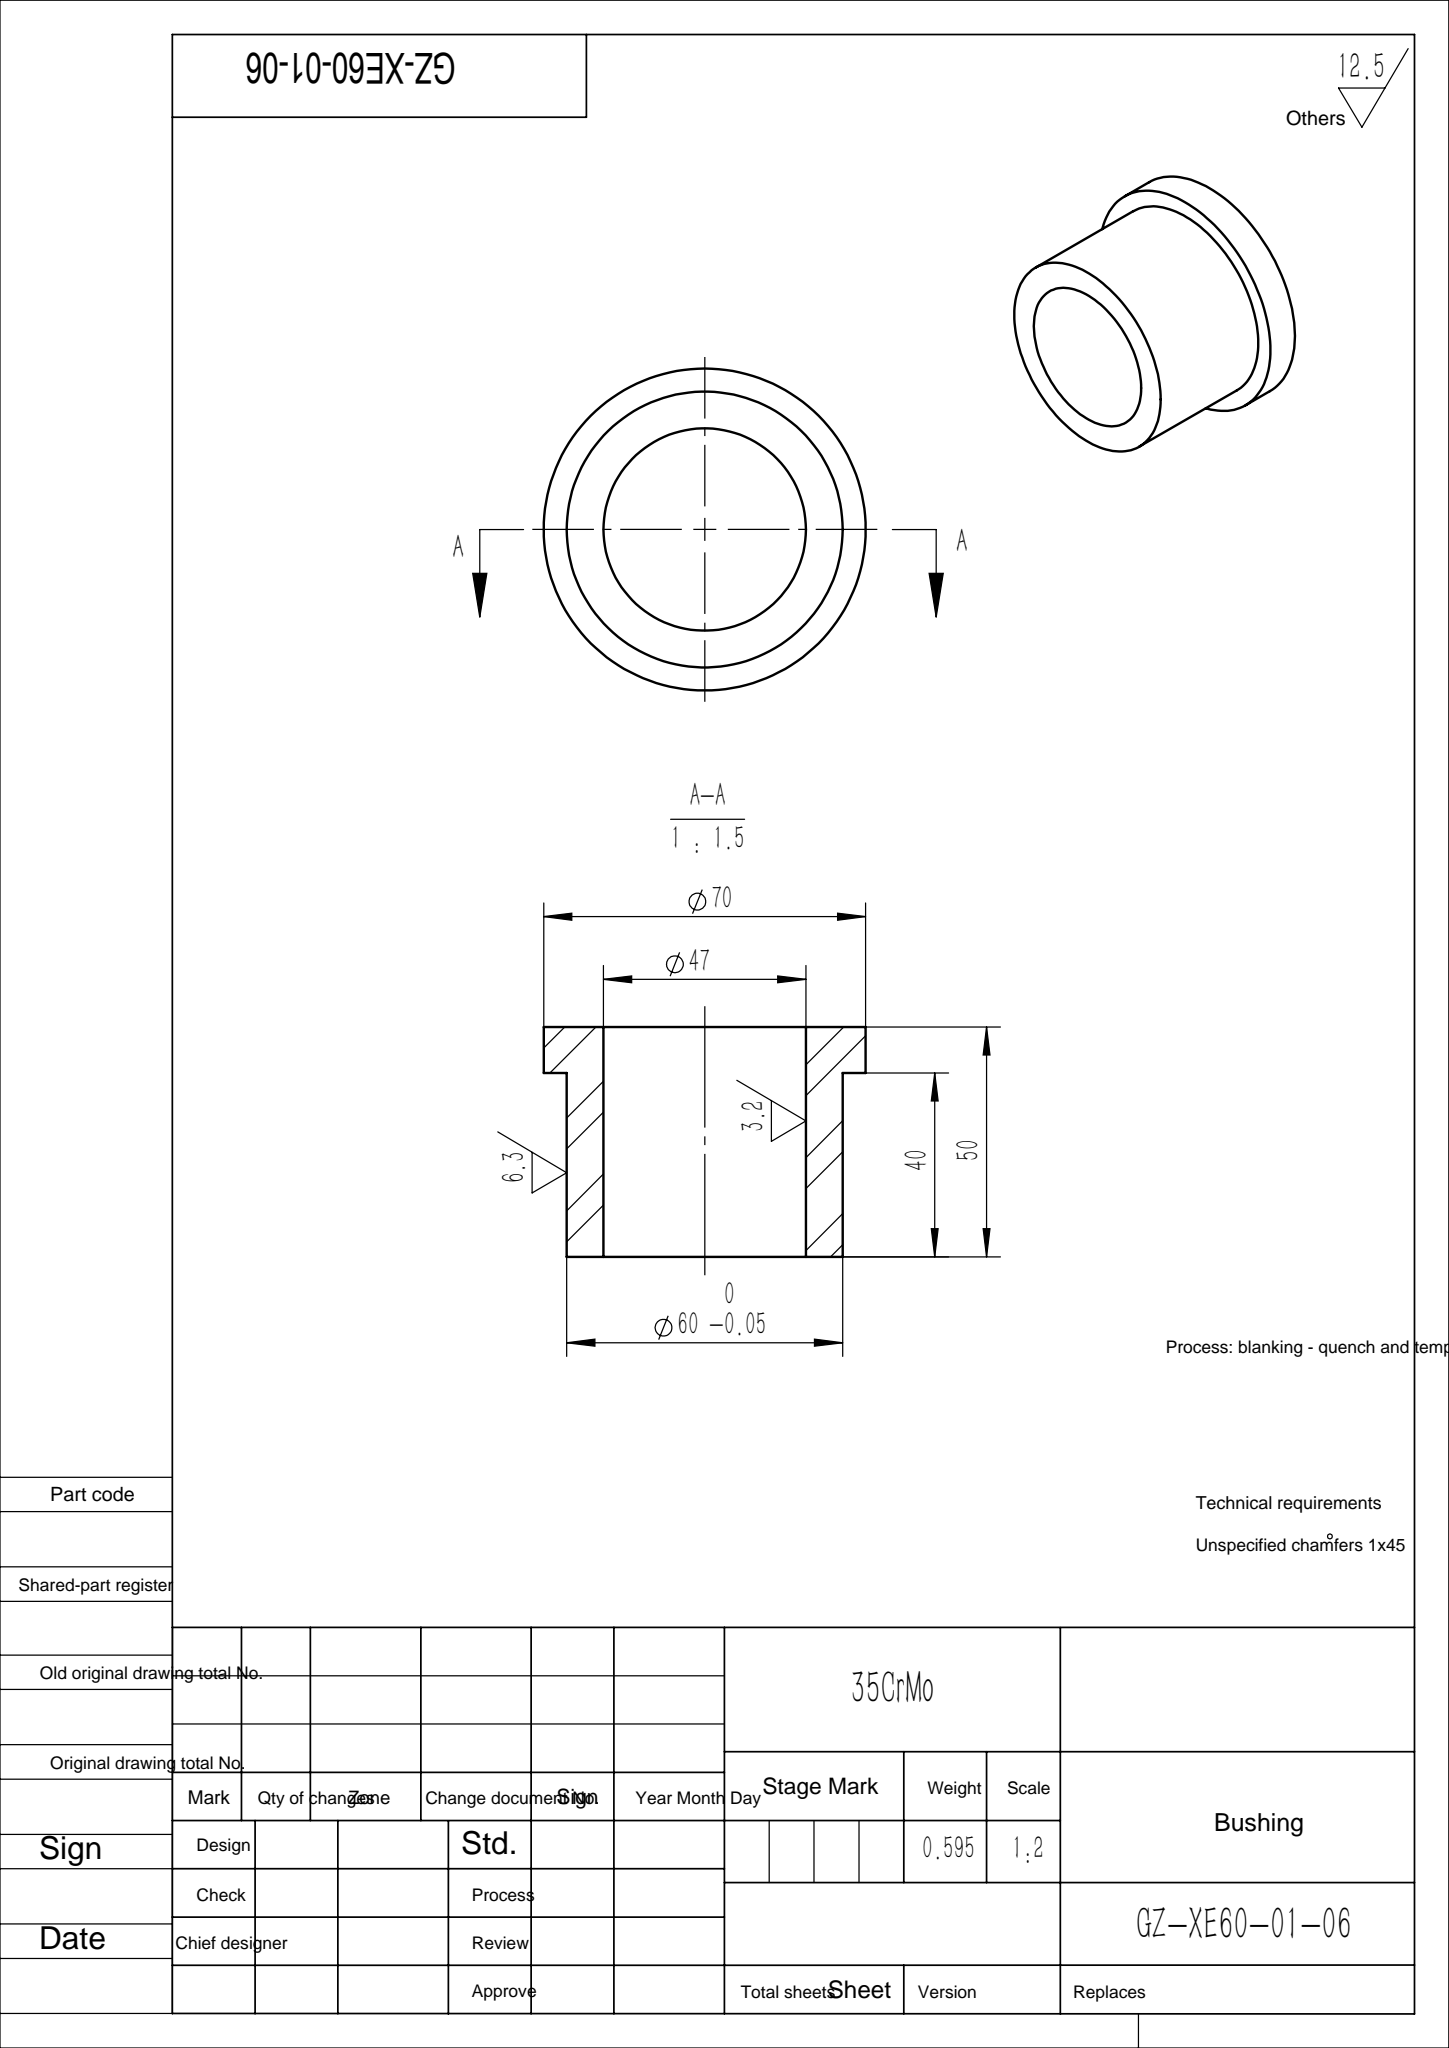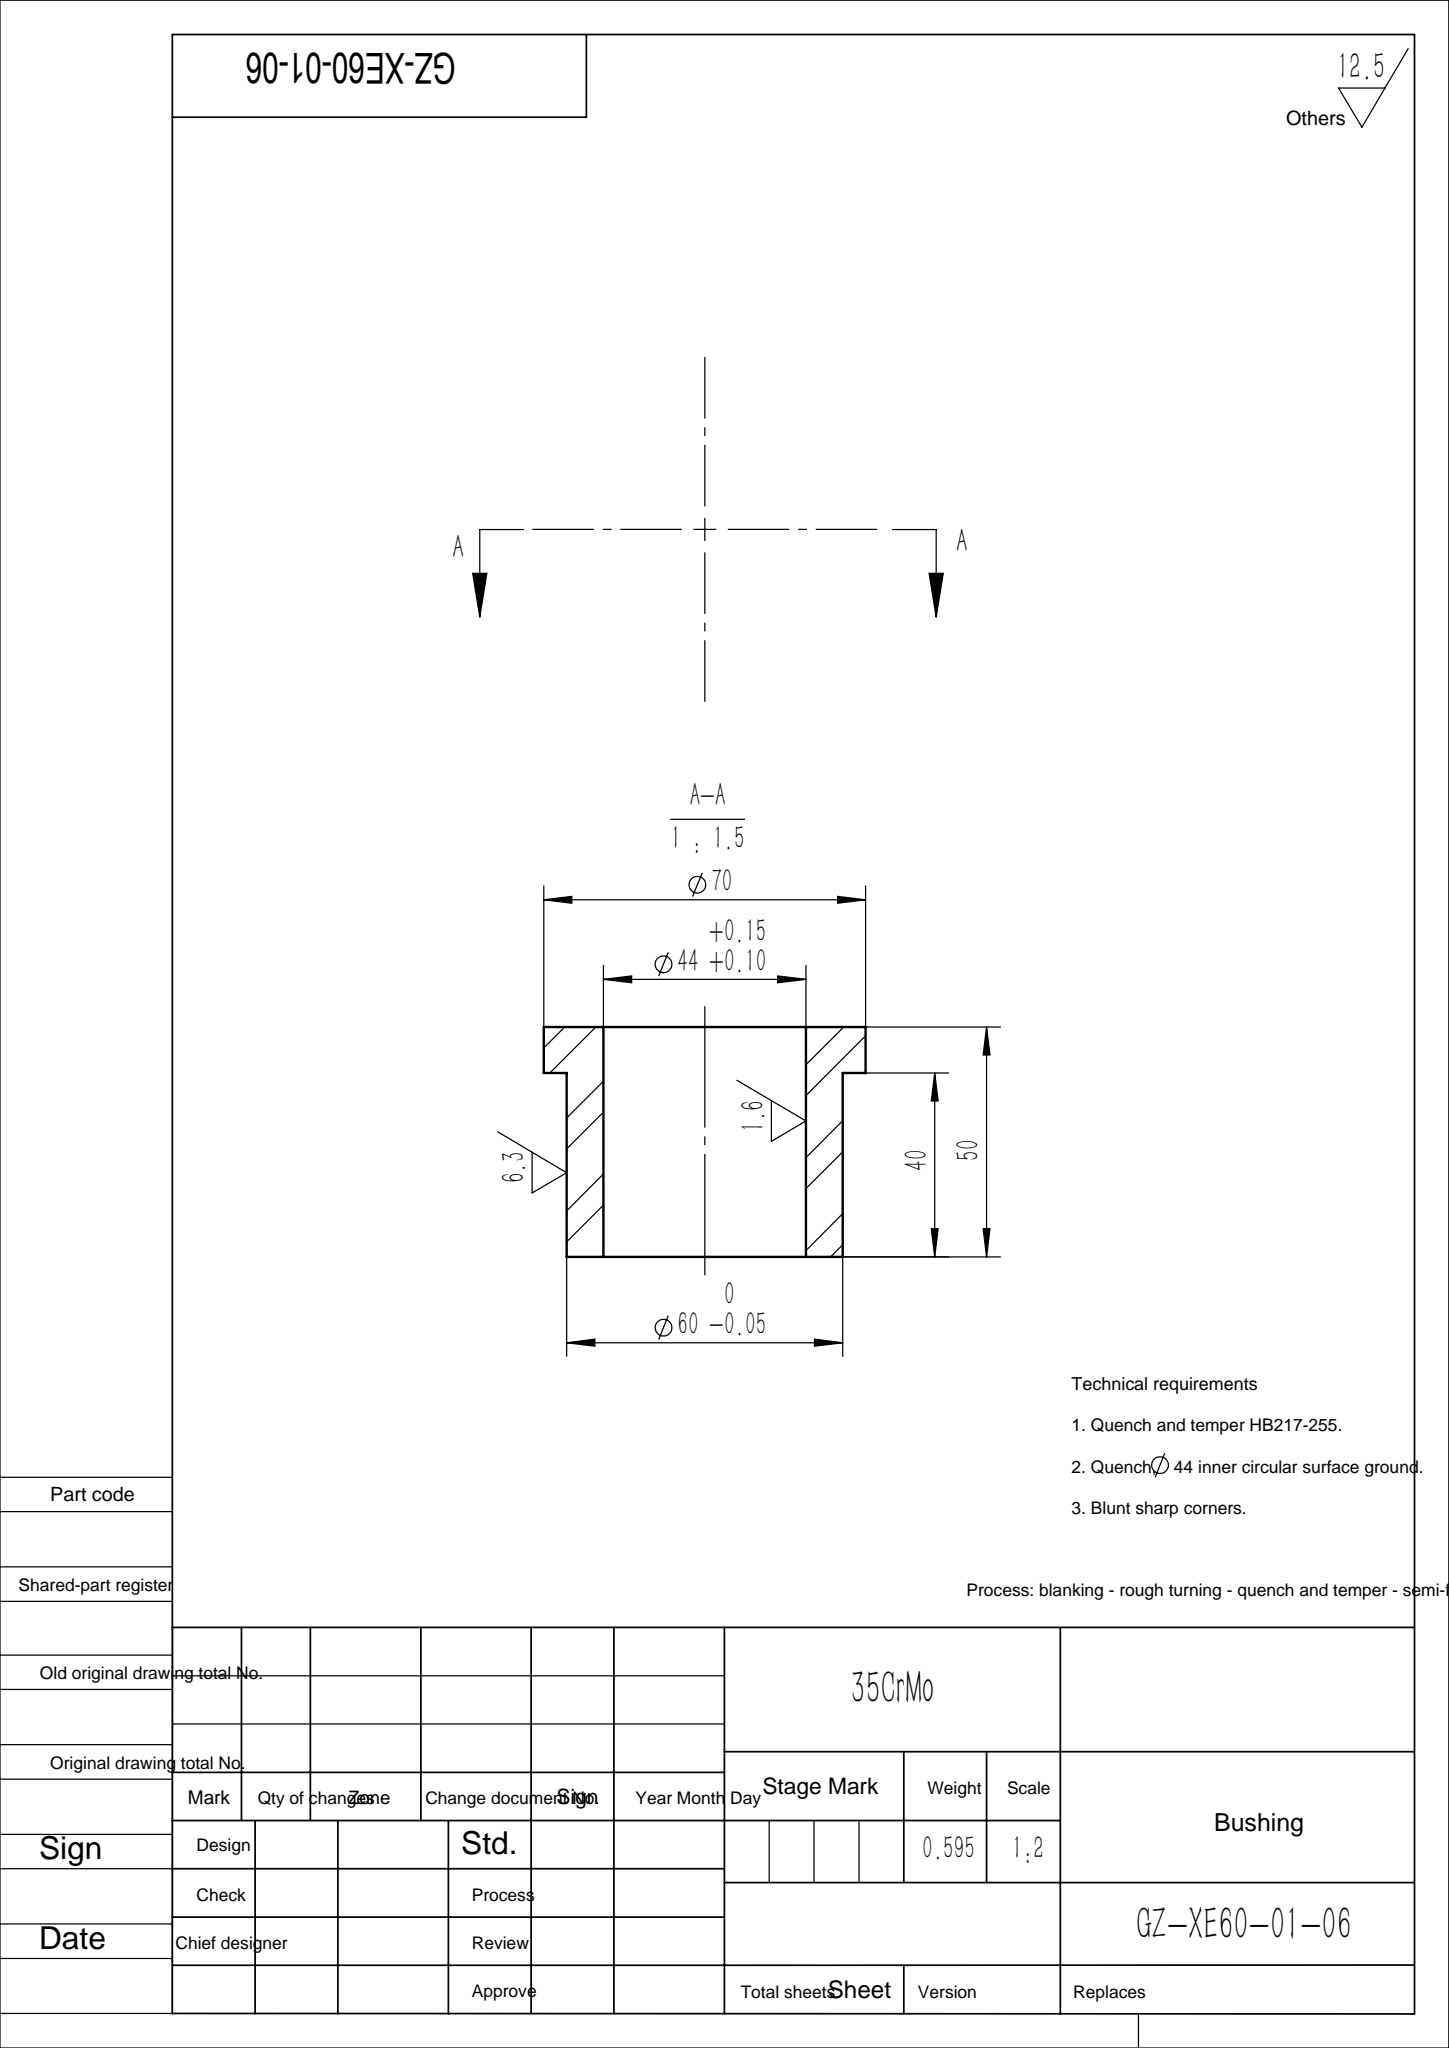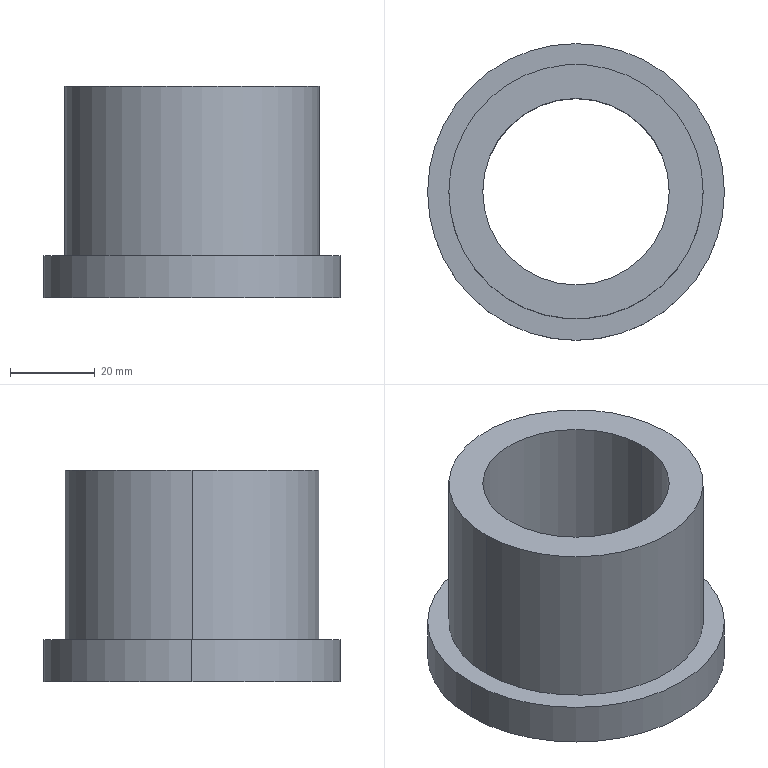Part | SolidWorks | features Extrusion 1, ICE 1 | 1 solid | 9 faces | box 70 x 70 x 50 mm | volume 75555 mm3 | cylinder 6 | plane 3 | commonest cylinder face diameters 44 x2 60 x2 70 x2
STEP:
#1=CARTESIAN_POINT('',(-35.,0.,-10.));
#2=VERTEX_POINT('',#1);
#3=CARTESIAN_POINT('',(35.,0.,-10.));
#4=VERTEX_POINT('',#3);
#5=CARTESIAN_POINT('',(0.,0.,-10.));
#6=DIRECTION('',(0.,0.,-1.));
#7=DIRECTION('',(-1.,0.,0.));
#8=AXIS2_PLACEMENT_3D('',#5,#6,#7);
#9=CIRCLE('',#8,35.);
#10=EDGE_CURVE('',#2,#4,#9,.T.);
#11=ORIENTED_EDGE('',*,*,#10,.F.);
#12=CARTESIAN_POINT('',(-35.,0.,0.));
#13=VERTEX_POINT('',#12);
#14=CARTESIAN_POINT('',(-35.,0.,-10.));
#15=DIRECTION('',(0.,0.,1.));
#16=VECTOR('',#15,1000.);
#17=LINE('',#14,#16);
#18=EDGE_CURVE('',#2,#13,#17,.T.);
#19=ORIENTED_EDGE('',*,*,#18,.T.);
#20=CARTESIAN_POINT('',(35.,0.,0.));
#21=VERTEX_POINT('',#20);
#22=CARTESIAN_POINT('',(0.,0.,0.));
#23=DIRECTION('',(0.,0.,-1.));
#24=DIRECTION('',(-1.,0.,0.));
#25=AXIS2_PLACEMENT_3D('',#22,#23,#24);
#26=CIRCLE('',#25,35.);
#27=EDGE_CURVE('',#13,#21,#26,.T.);
#28=ORIENTED_EDGE('',*,*,#27,.T.);
#29=CARTESIAN_POINT('',(35.,0.,-10.));
#30=DIRECTION('',(0.,0.,1.));
#31=VECTOR('',#30,1000.);
#32=LINE('',#29,#31);
#33=EDGE_CURVE('',#4,#21,#32,.T.);
#34=ORIENTED_EDGE('',*,*,#33,.F.);
#35=EDGE_LOOP('',(#11,#19,#28,#34));
#36=FACE_OUTER_BOUND('',#35,.T.);
#37=CARTESIAN_POINT('',(0.,0.,-10.));
#38=DIRECTION('',(0.,0.,1.));
#39=DIRECTION('',(1.,0.,0.));
#40=AXIS2_PLACEMENT_3D('',#37,#38,#39);
#41=CYLINDRICAL_SURFACE('',#40,35.);
#42=ADVANCED_FACE('',(#36),#41,.T.);
#43=CARTESIAN_POINT('',(-22.,0.,40.));
#44=VERTEX_POINT('',#43);
#45=CARTESIAN_POINT('',(22.,0.,40.));
#46=VERTEX_POINT('',#45);
#47=CARTESIAN_POINT('',(0.,0.,40.));
#48=DIRECTION('',(0.,0.,1.));
#49=DIRECTION('',(1.,0.,0.));
#50=AXIS2_PLACEMENT_3D('',#47,#48,#49);
#51=CIRCLE('',#50,22.);
#52=EDGE_CURVE('',#44,#46,#51,.T.);
#53=ORIENTED_EDGE('',*,*,#52,.T.);
#54=CARTESIAN_POINT('',(22.,0.,-10.));
#55=VERTEX_POINT('',#54);
#56=CARTESIAN_POINT('',(22.,0.,40.));
#57=DIRECTION('',(0.,0.,-1.));
#58=VECTOR('',#57,1000.);
#59=LINE('',#56,#58);
#60=EDGE_CURVE('',#46,#55,#59,.T.);
#61=ORIENTED_EDGE('',*,*,#60,.T.);
#62=CARTESIAN_POINT('',(-22.,0.,-10.));
#63=VERTEX_POINT('',#62);
#64=CARTESIAN_POINT('',(0.,0.,-10.));
#65=DIRECTION('',(0.,0.,-1.));
#66=DIRECTION('',(-1.,0.,0.));
#67=AXIS2_PLACEMENT_3D('',#64,#65,#66);
#68=CIRCLE('',#67,22.);
#69=EDGE_CURVE('',#55,#63,#68,.T.);
#70=ORIENTED_EDGE('',*,*,#69,.T.);
#71=CARTESIAN_POINT('',(-22.,0.,40.));
#72=DIRECTION('',(0.,0.,-1.));
#73=VECTOR('',#72,1000.);
#74=LINE('',#71,#73);
#75=EDGE_CURVE('',#44,#63,#74,.T.);
#76=ORIENTED_EDGE('',*,*,#75,.F.);
#77=EDGE_LOOP('',(#53,#61,#70,#76));
#78=FACE_OUTER_BOUND('',#77,.T.);
#79=CARTESIAN_POINT('',(0.,0.,40.));
#80=DIRECTION('',(0.,0.,-1.));
#81=DIRECTION('',(-1.,0.,0.));
#82=AXIS2_PLACEMENT_3D('',#79,#80,#81);
#83=CYLINDRICAL_SURFACE('',#82,22.);
#84=ADVANCED_FACE('',(#78),#83,.F.);
#85=CARTESIAN_POINT('',(30.,0.,40.));
#86=VERTEX_POINT('',#85);
#87=CARTESIAN_POINT('',(-30.,0.,40.));
#88=VERTEX_POINT('',#87);
#89=CARTESIAN_POINT('',(0.,0.,40.));
#90=DIRECTION('',(0.,0.,1.));
#91=DIRECTION('',(1.,0.,0.));
#92=AXIS2_PLACEMENT_3D('',#89,#90,#91);
#93=CIRCLE('',#92,30.);
#94=EDGE_CURVE('',#86,#88,#93,.T.);
#95=ORIENTED_EDGE('',*,*,#94,.F.);
#96=CARTESIAN_POINT('',(30.,0.,0.));
#97=VERTEX_POINT('',#96);
#98=CARTESIAN_POINT('',(30.,0.,40.));
#99=DIRECTION('',(0.,0.,-1.));
#100=VECTOR('',#99,1000.);
#101=LINE('',#98,#100);
#102=EDGE_CURVE('',#86,#97,#101,.T.);
#103=ORIENTED_EDGE('',*,*,#102,.T.);
#104=CARTESIAN_POINT('',(-30.,0.,0.));
#105=VERTEX_POINT('',#104);
#106=CARTESIAN_POINT('',(0.,0.,0.));
#107=DIRECTION('',(0.,0.,-1.));
#108=DIRECTION('',(-1.,0.,0.));
#109=AXIS2_PLACEMENT_3D('',#106,#107,#108);
#110=CIRCLE('',#109,30.);
#111=EDGE_CURVE('',#105,#97,#110,.T.);
#112=ORIENTED_EDGE('',*,*,#111,.F.);
#113=CARTESIAN_POINT('',(-30.,0.,40.));
#114=DIRECTION('',(0.,0.,-1.));
#115=VECTOR('',#114,1000.);
#116=LINE('',#113,#115);
#117=EDGE_CURVE('',#88,#105,#116,.T.);
#118=ORIENTED_EDGE('',*,*,#117,.F.);
#119=EDGE_LOOP('',(#95,#103,#112,#118));
#120=FACE_OUTER_BOUND('',#119,.T.);
#121=CARTESIAN_POINT('',(0.,0.,40.));
#122=DIRECTION('',(0.,0.,-1.));
#123=DIRECTION('',(-1.,0.,0.));
#124=AXIS2_PLACEMENT_3D('',#121,#122,#123);
#125=CYLINDRICAL_SURFACE('',#124,30.);
#126=ADVANCED_FACE('',(#120),#125,.T.);
#127=CARTESIAN_POINT('',(0.,0.,40.));
#128=DIRECTION('',(0.,0.,1.));
#129=DIRECTION('',(1.,0.,0.));
#130=AXIS2_PLACEMENT_3D('',#127,#128,#129);
#131=CIRCLE('',#130,30.);
#132=EDGE_CURVE('',#88,#86,#131,.T.);
#133=ORIENTED_EDGE('',*,*,#132,.T.);
#134=ORIENTED_EDGE('',*,*,#94,.T.);
#135=EDGE_LOOP('',(#133,#134));
#136=FACE_OUTER_BOUND('',#135,.T.);
#137=ORIENTED_EDGE('',*,*,#52,.F.);
#138=CARTESIAN_POINT('',(0.,0.,40.));
#139=DIRECTION('',(0.,0.,1.));
#140=DIRECTION('',(1.,0.,0.));
#141=AXIS2_PLACEMENT_3D('',#138,#139,#140);
#142=CIRCLE('',#141,22.);
#143=EDGE_CURVE('',#46,#44,#142,.T.);
#144=ORIENTED_EDGE('',*,*,#143,.F.);
#145=EDGE_LOOP('',(#137,#144));
#146=FACE_BOUND('',#145,.T.);
#147=CARTESIAN_POINT('',(0.,0.,40.));
#148=DIRECTION('',(0.,0.,1.));
#149=DIRECTION('',(1.,0.,0.));
#150=AXIS2_PLACEMENT_3D('',#147,#148,#149);
#151=PLANE('',#150);
#152=ADVANCED_FACE('',(#136,#146),#151,.T.);
#153=ORIENTED_EDGE('',*,*,#102,.F.);
#154=ORIENTED_EDGE('',*,*,#132,.F.);
#155=ORIENTED_EDGE('',*,*,#117,.T.);
#156=CARTESIAN_POINT('',(0.,0.,0.));
#157=DIRECTION('',(0.,0.,-1.));
#158=DIRECTION('',(-1.,0.,0.));
#159=AXIS2_PLACEMENT_3D('',#156,#157,#158);
#160=CIRCLE('',#159,30.);
#161=EDGE_CURVE('',#97,#105,#160,.T.);
#162=ORIENTED_EDGE('',*,*,#161,.F.);
#163=EDGE_LOOP('',(#153,#154,#155,#162));
#164=FACE_OUTER_BOUND('',#163,.T.);
#165=CARTESIAN_POINT('',(0.,0.,40.));
#166=DIRECTION('',(0.,0.,-1.));
#167=DIRECTION('',(-1.,0.,0.));
#168=AXIS2_PLACEMENT_3D('',#165,#166,#167);
#169=CYLINDRICAL_SURFACE('',#168,30.);
#170=ADVANCED_FACE('',(#164),#169,.T.);
#171=ORIENTED_EDGE('',*,*,#60,.F.);
#172=ORIENTED_EDGE('',*,*,#143,.T.);
#173=ORIENTED_EDGE('',*,*,#75,.T.);
#174=CARTESIAN_POINT('',(0.,0.,-10.));
#175=DIRECTION('',(0.,0.,-1.));
#176=DIRECTION('',(-1.,0.,0.));
#177=AXIS2_PLACEMENT_3D('',#174,#175,#176);
#178=CIRCLE('',#177,22.);
#179=EDGE_CURVE('',#63,#55,#178,.T.);
#180=ORIENTED_EDGE('',*,*,#179,.T.);
#181=EDGE_LOOP('',(#171,#172,#173,#180));
#182=FACE_OUTER_BOUND('',#181,.T.);
#183=CARTESIAN_POINT('',(0.,0.,40.));
#184=DIRECTION('',(0.,0.,-1.));
#185=DIRECTION('',(-1.,0.,0.));
#186=AXIS2_PLACEMENT_3D('',#183,#184,#185);
#187=CYLINDRICAL_SURFACE('',#186,22.);
#188=ADVANCED_FACE('',(#182),#187,.F.);
#189=CARTESIAN_POINT('',(0.,0.,0.));
#190=DIRECTION('',(0.,0.,-1.));
#191=DIRECTION('',(-1.,0.,0.));
#192=AXIS2_PLACEMENT_3D('',#189,#190,#191);
#193=CIRCLE('',#192,35.);
#194=EDGE_CURVE('',#21,#13,#193,.T.);
#195=ORIENTED_EDGE('',*,*,#194,.F.);
#196=ORIENTED_EDGE('',*,*,#27,.F.);
#197=EDGE_LOOP('',(#195,#196));
#198=FACE_OUTER_BOUND('',#197,.T.);
#199=ORIENTED_EDGE('',*,*,#111,.T.);
#200=ORIENTED_EDGE('',*,*,#161,.T.);
#201=EDGE_LOOP('',(#199,#200));
#202=FACE_BOUND('',#201,.T.);
#203=CARTESIAN_POINT('',(0.,0.,0.));
#204=DIRECTION('',(0.,0.,-1.));
#205=DIRECTION('',(-1.,0.,0.));
#206=AXIS2_PLACEMENT_3D('',#203,#204,#205);
#207=PLANE('',#206);
#208=ADVANCED_FACE('',(#198,#202),#207,.F.);
#209=CARTESIAN_POINT('',(0.,0.,-10.));
#210=DIRECTION('',(0.,0.,-1.));
#211=DIRECTION('',(-1.,0.,0.));
#212=AXIS2_PLACEMENT_3D('',#209,#210,#211);
#213=CIRCLE('',#212,35.);
#214=EDGE_CURVE('',#4,#2,#213,.T.);
#215=ORIENTED_EDGE('',*,*,#214,.T.);
#216=ORIENTED_EDGE('',*,*,#10,.T.);
#217=EDGE_LOOP('',(#215,#216));
#218=FACE_OUTER_BOUND('',#217,.T.);
#219=ORIENTED_EDGE('',*,*,#179,.F.);
#220=ORIENTED_EDGE('',*,*,#69,.F.);
#221=EDGE_LOOP('',(#219,#220));
#222=FACE_BOUND('',#221,.T.);
#223=CARTESIAN_POINT('',(0.,0.,-10.));
#224=DIRECTION('',(0.,0.,-1.));
#225=DIRECTION('',(-1.,0.,0.));
#226=AXIS2_PLACEMENT_3D('',#223,#224,#225);
#227=PLANE('',#226);
#228=ADVANCED_FACE('',(#218,#222),#227,.T.);
#229=ORIENTED_EDGE('',*,*,#18,.F.);
#230=ORIENTED_EDGE('',*,*,#214,.F.);
#231=ORIENTED_EDGE('',*,*,#33,.T.);
#232=ORIENTED_EDGE('',*,*,#194,.T.);
#233=EDGE_LOOP('',(#229,#230,#231,#232));
#234=FACE_OUTER_BOUND('',#233,.T.);
#235=CARTESIAN_POINT('',(0.,0.,-10.));
#236=DIRECTION('',(0.,0.,1.));
#237=DIRECTION('',(1.,0.,0.));
#238=AXIS2_PLACEMENT_3D('',#235,#236,#237);
#239=CYLINDRICAL_SURFACE('',#238,35.);
#240=ADVANCED_FACE('',(#234),#239,.T.);
#241=CLOSED_SHELL('',(#42,#84,#126,#152,#170,#188,#208,#228,#240));
#242=MANIFOLD_SOLID_BREP('',#241);
#243=CARTESIAN_POINT('',(0.,0.,0.));
#244=DIRECTION('',(0.,0.,1.));
#245=DIRECTION('',(1.,0.,0.));
#246=AXIS2_PLACEMENT_3D('',#243,#244,#245);
#247=(LENGTH_UNIT()NAMED_UNIT(*)SI_UNIT(.MILLI.,.METRE.));
#248=UNCERTAINTY_MEASURE_WITH_UNIT(LENGTH_MEASURE(0.00001),#247,'','');
#249=(NAMED_UNIT(*)PLANE_ANGLE_UNIT()SI_UNIT($,.RADIAN.));
#250=(NAMED_UNIT(*)SI_UNIT($,.STERADIAN.)SOLID_ANGLE_UNIT());
#251=(GEOMETRIC_REPRESENTATION_CONTEXT(3)GLOBAL_UNCERTAINTY_ASSIGNED_CONTEXT((#248))GLOBAL_UNIT_ASSIGNED_CONTEXT((#247,#249,#250))REPRESENTATION_CONTEXT('',''));
#252=ADVANCED_BREP_SHAPE_REPRESENTATION('',(#242,#246),#251);